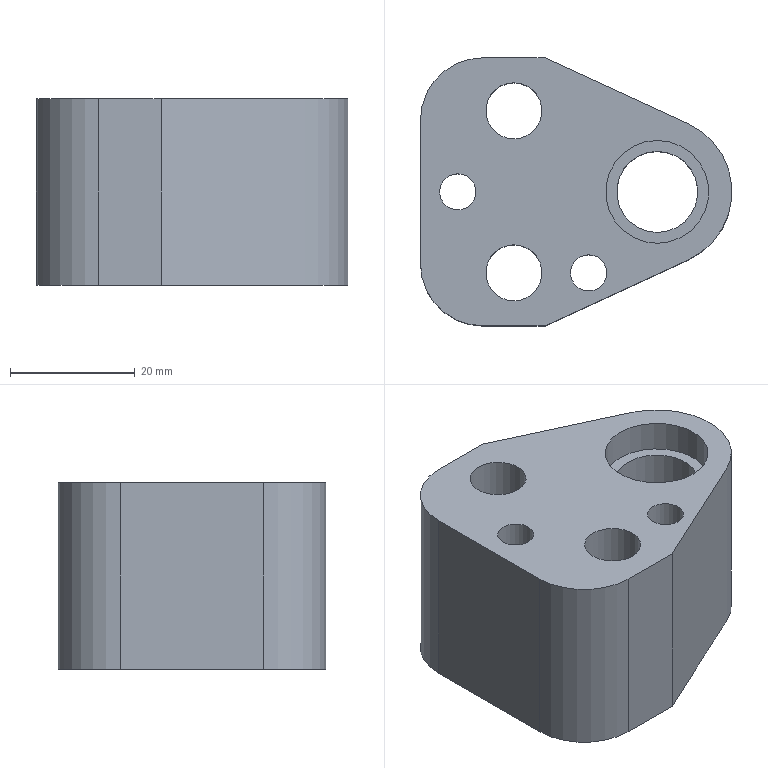Part | NX | features solid 2 | 1 solid | 27 faces | box 50 x 43 x 30 mm | volume 37617 mm3 | plane 14 | cylinder 13 | commonest cylinder face diameters 5.8 x2 8 x2 9 x2 14 x2 20 x2 13 x1
STEP:
#1=CARTESIAN_POINT('',(344.165,-485.402,142.));
#2=VERTEX_POINT('',#1);
#3=CARTESIAN_POINT('',(344.165,-485.402,172.));
#4=VERTEX_POINT('',#3);
#5=CARTESIAN_POINT('',(344.165,-485.402,142.));
#6=DIRECTION('',(0.,0.,1.));
#7=VECTOR('',#6,1000.);
#8=LINE('',#5,#7);
#9=EDGE_CURVE('',#2,#4,#8,.T.);
#10=ORIENTED_EDGE('',*,*,#9,.F.);
#11=CARTESIAN_POINT('',(344.165,-485.402,142.));
#12=VERTEX_POINT('',#11);
#13=CARTESIAN_POINT('',(344.165,-474.502,142.));
#14=DIRECTION('',(0.,1.,0.));
#15=VECTOR('',#14,1000.);
#16=LINE('',#13,#15);
#17=EDGE_CURVE('',#2,#12,#16,.T.);
#18=ORIENTED_EDGE('',*,*,#17,.T.);
#19=CARTESIAN_POINT('',(344.165,-485.402,172.));
#20=VERTEX_POINT('',#19);
#21=CARTESIAN_POINT('',(344.165,-485.402,172.));
#22=DIRECTION('',(0.,0.,-1.));
#23=VECTOR('',#22,1000.);
#24=LINE('',#21,#23);
#25=EDGE_CURVE('',#20,#12,#24,.T.);
#26=ORIENTED_EDGE('',*,*,#25,.F.);
#27=CARTESIAN_POINT('',(344.165,-474.502,172.));
#28=DIRECTION('',(0.,-1.,0.));
#29=VECTOR('',#28,1000.);
#30=LINE('',#27,#29);
#31=EDGE_CURVE('',#20,#4,#30,.T.);
#32=ORIENTED_EDGE('',*,*,#31,.T.);
#33=EDGE_LOOP('',(#10,#18,#26,#32));
#34=FACE_BOUND('',#33,.T.);
#35=CARTESIAN_POINT('',(344.165,-474.502,142.));
#36=DIRECTION('',(1.,0.,0.));
#37=DIRECTION('',(0.,0.,1.));
#38=AXIS2_PLACEMENT_3D('',#35,#36,#37);
#39=PLANE('',#38);
#40=ADVANCED_FACE('',(#34),#39,.T.);
#41=CARTESIAN_POINT('',(321.145,-496.002,172.));
#42=VERTEX_POINT('',#41);
#43=CARTESIAN_POINT('',(339.311,-487.637,172.));
#44=DIRECTION('',(0.9083,0.4183,0.));
#45=VECTOR('',#44,1000.);
#46=LINE('',#43,#45);
#47=EDGE_CURVE('',#42,#4,#46,.T.);
#48=ORIENTED_EDGE('',*,*,#47,.T.);
#49=ORIENTED_EDGE('',*,*,#31,.F.);
#50=CARTESIAN_POINT('',(344.165,-463.603,172.));
#51=VERTEX_POINT('',#50);
#52=CARTESIAN_POINT('',(339.145,-474.502,172.));
#53=DIRECTION('',(0.,0.,-1.));
#54=DIRECTION('',(0.,1.,0.));
#55=AXIS2_PLACEMENT_3D('',#52,#53,#54);
#56=CIRCLE('',#55,12.);
#57=EDGE_CURVE('',#51,#20,#56,.T.);
#58=ORIENTED_EDGE('',*,*,#57,.F.);
#59=CARTESIAN_POINT('',(344.165,-463.603,172.));
#60=VERTEX_POINT('',#59);
#61=CARTESIAN_POINT('',(344.165,-474.502,172.));
#62=DIRECTION('',(0.,-1.,0.));
#63=VECTOR('',#62,1000.);
#64=LINE('',#61,#63);
#65=EDGE_CURVE('',#60,#51,#64,.T.);
#66=ORIENTED_EDGE('',*,*,#65,.F.);
#67=CARTESIAN_POINT('',(321.145,-453.002,172.));
#68=VERTEX_POINT('',#67);
#69=CARTESIAN_POINT('',(339.311,-461.368,172.));
#70=DIRECTION('',(-0.9083,0.4183,0.));
#71=VECTOR('',#70,1000.);
#72=LINE('',#69,#71);
#73=EDGE_CURVE('',#60,#68,#72,.T.);
#74=ORIENTED_EDGE('',*,*,#73,.T.);
#75=CARTESIAN_POINT('',(311.145,-453.002,172.));
#76=VERTEX_POINT('',#75);
#77=CARTESIAN_POINT('',(332.655,-453.002,172.));
#78=DIRECTION('',(1.,0.,0.));
#79=VECTOR('',#78,1000.);
#80=LINE('',#77,#79);
#81=EDGE_CURVE('',#76,#68,#80,.T.);
#82=ORIENTED_EDGE('',*,*,#81,.F.);
#83=CARTESIAN_POINT('',(301.145,-463.002,172.));
#84=VERTEX_POINT('',#83);
#85=CARTESIAN_POINT('',(311.145,-463.002,172.));
#86=DIRECTION('',(0.,0.,1.));
#87=DIRECTION('',(0.,-1.,0.));
#88=AXIS2_PLACEMENT_3D('',#85,#86,#87);
#89=CIRCLE('',#88,10.);
#90=EDGE_CURVE('',#76,#84,#89,.T.);
#91=ORIENTED_EDGE('',*,*,#90,.T.);
#92=CARTESIAN_POINT('',(301.145,-486.002,172.));
#93=VERTEX_POINT('',#92);
#94=CARTESIAN_POINT('',(301.145,-474.502,172.));
#95=DIRECTION('',(0.,1.,0.));
#96=VECTOR('',#95,1000.);
#97=LINE('',#94,#96);
#98=EDGE_CURVE('',#93,#84,#97,.T.);
#99=ORIENTED_EDGE('',*,*,#98,.F.);
#100=CARTESIAN_POINT('',(311.145,-496.002,172.));
#101=VERTEX_POINT('',#100);
#102=CARTESIAN_POINT('',(311.145,-486.002,172.));
#103=DIRECTION('',(0.,0.,1.));
#104=DIRECTION('',(0.,-1.,0.));
#105=AXIS2_PLACEMENT_3D('',#102,#103,#104);
#106=CIRCLE('',#105,10.);
#107=EDGE_CURVE('',#93,#101,#106,.T.);
#108=ORIENTED_EDGE('',*,*,#107,.T.);
#109=CARTESIAN_POINT('',(332.655,-496.002,172.));
#110=DIRECTION('',(-1.,0.,0.));
#111=VECTOR('',#110,1000.);
#112=LINE('',#109,#111);
#113=EDGE_CURVE('',#42,#101,#112,.T.);
#114=ORIENTED_EDGE('',*,*,#113,.F.);
#115=EDGE_LOOP('',(#48,#49,#58,#66,#74,#82,#91,#99,#108,#114));
#116=FACE_BOUND('',#115,.T.);
#117=CARTESIAN_POINT('',(307.145,-471.602,172.));
#118=VERTEX_POINT('',#117);
#119=CARTESIAN_POINT('',(307.145,-474.502,172.));
#120=DIRECTION('',(0.,0.,-1.));
#121=DIRECTION('',(0.,1.,0.));
#122=AXIS2_PLACEMENT_3D('',#119,#120,#121);
#123=CIRCLE('',#122,2.9);
#124=EDGE_CURVE('',#118,#118,#123,.T.);
#125=ORIENTED_EDGE('',*,*,#124,.T.);
#126=EDGE_LOOP('',(#125));
#127=FACE_BOUND('',#126,.T.);
#128=CARTESIAN_POINT('',(328.145,-484.602,172.));
#129=VERTEX_POINT('',#128);
#130=CARTESIAN_POINT('',(328.145,-487.502,172.));
#131=DIRECTION('',(0.,0.,-1.));
#132=DIRECTION('',(0.,1.,0.));
#133=AXIS2_PLACEMENT_3D('',#130,#131,#132);
#134=CIRCLE('',#133,2.9);
#135=EDGE_CURVE('',#129,#129,#134,.T.);
#136=ORIENTED_EDGE('',*,*,#135,.T.);
#137=EDGE_LOOP('',(#136));
#138=FACE_BOUND('',#137,.T.);
#139=CARTESIAN_POINT('',(316.145,-483.002,172.));
#140=VERTEX_POINT('',#139);
#141=CARTESIAN_POINT('',(316.145,-487.502,172.));
#142=DIRECTION('',(0.,0.,-1.));
#143=DIRECTION('',(0.,1.,0.));
#144=AXIS2_PLACEMENT_3D('',#141,#142,#143);
#145=CIRCLE('',#144,4.5);
#146=EDGE_CURVE('',#140,#140,#145,.T.);
#147=ORIENTED_EDGE('',*,*,#146,.T.);
#148=EDGE_LOOP('',(#147));
#149=FACE_BOUND('',#148,.T.);
#150=CARTESIAN_POINT('',(316.145,-457.002,172.));
#151=VERTEX_POINT('',#150);
#152=CARTESIAN_POINT('',(316.145,-461.502,172.));
#153=DIRECTION('',(0.,0.,-1.));
#154=DIRECTION('',(0.,1.,0.));
#155=AXIS2_PLACEMENT_3D('',#152,#153,#154);
#156=CIRCLE('',#155,4.5);
#157=EDGE_CURVE('',#151,#151,#156,.T.);
#158=ORIENTED_EDGE('',*,*,#157,.T.);
#159=EDGE_LOOP('',(#158));
#160=FACE_BOUND('',#159,.T.);
#161=CARTESIAN_POINT('',(339.145,-466.252,172.));
#162=VERTEX_POINT('',#161);
#163=CARTESIAN_POINT('',(339.145,-474.502,172.));
#164=DIRECTION('',(0.,0.,-1.));
#165=DIRECTION('',(0.,1.,0.));
#166=AXIS2_PLACEMENT_3D('',#163,#164,#165);
#167=CIRCLE('',#166,8.25);
#168=EDGE_CURVE('',#162,#162,#167,.T.);
#169=ORIENTED_EDGE('',*,*,#168,.T.);
#170=EDGE_LOOP('',(#169));
#171=FACE_BOUND('',#170,.T.);
#172=CARTESIAN_POINT('',(332.655,-474.502,172.));
#173=DIRECTION('',(0.,0.,1.));
#174=DIRECTION('',(0.,-1.,0.));
#175=AXIS2_PLACEMENT_3D('',#172,#173,#174);
#176=PLANE('',#175);
#177=ADVANCED_FACE('',(#116,#127,#138,#149,#160,#171),#176,.T.);
#178=CARTESIAN_POINT('',(321.145,-453.002,142.));
#179=VERTEX_POINT('',#178);
#180=CARTESIAN_POINT('',(321.145,-453.002,142.));
#181=DIRECTION('',(0.,0.,1.));
#182=VECTOR('',#181,1000.);
#183=LINE('',#180,#182);
#184=EDGE_CURVE('',#179,#68,#183,.T.);
#185=ORIENTED_EDGE('',*,*,#184,.F.);
#186=CARTESIAN_POINT('',(311.145,-453.002,142.));
#187=VERTEX_POINT('',#186);
#188=CARTESIAN_POINT('',(332.655,-453.002,142.));
#189=DIRECTION('',(-1.,0.,0.));
#190=VECTOR('',#189,1000.);
#191=LINE('',#188,#190);
#192=EDGE_CURVE('',#179,#187,#191,.T.);
#193=ORIENTED_EDGE('',*,*,#192,.T.);
#194=CARTESIAN_POINT('',(311.145,-453.002,142.));
#195=DIRECTION('',(0.,0.,1.));
#196=VECTOR('',#195,1000.);
#197=LINE('',#194,#196);
#198=EDGE_CURVE('',#187,#76,#197,.T.);
#199=ORIENTED_EDGE('',*,*,#198,.T.);
#200=ORIENTED_EDGE('',*,*,#81,.T.);
#201=EDGE_LOOP('',(#185,#193,#199,#200));
#202=FACE_BOUND('',#201,.T.);
#203=CARTESIAN_POINT('',(332.655,-453.002,142.));
#204=DIRECTION('',(0.,1.,0.));
#205=DIRECTION('',(0.,0.,1.));
#206=AXIS2_PLACEMENT_3D('',#203,#204,#205);
#207=PLANE('',#206);
#208=ADVANCED_FACE('',(#202),#207,.T.);
#209=CARTESIAN_POINT('',(344.165,-463.603,142.));
#210=VERTEX_POINT('',#209);
#211=CARTESIAN_POINT('',(344.165,-463.603,142.));
#212=DIRECTION('',(0.,0.,-1.));
#213=VECTOR('',#212,1000.);
#214=LINE('',#211,#213);
#215=EDGE_CURVE('',#60,#210,#214,.T.);
#216=ORIENTED_EDGE('',*,*,#215,.F.);
#217=ORIENTED_EDGE('',*,*,#65,.T.);
#218=CARTESIAN_POINT('',(344.165,-463.603,142.));
#219=VERTEX_POINT('',#218);
#220=CARTESIAN_POINT('',(344.165,-463.603,172.));
#221=DIRECTION('',(0.,0.,-1.));
#222=VECTOR('',#221,1000.);
#223=LINE('',#220,#222);
#224=EDGE_CURVE('',#219,#51,#223,.F.);
#225=ORIENTED_EDGE('',*,*,#224,.F.);
#226=CARTESIAN_POINT('',(344.165,-474.502,142.));
#227=DIRECTION('',(0.,1.,0.));
#228=VECTOR('',#227,1000.);
#229=LINE('',#226,#228);
#230=EDGE_CURVE('',#219,#210,#229,.T.);
#231=ORIENTED_EDGE('',*,*,#230,.T.);
#232=EDGE_LOOP('',(#216,#217,#225,#231));
#233=FACE_BOUND('',#232,.T.);
#234=CARTESIAN_POINT('',(344.165,-474.502,142.));
#235=DIRECTION('',(1.,0.,0.));
#236=DIRECTION('',(0.,0.,1.));
#237=AXIS2_PLACEMENT_3D('',#234,#235,#236);
#238=PLANE('',#237);
#239=ADVANCED_FACE('',(#233),#238,.T.);
#240=CARTESIAN_POINT('',(321.145,-496.002,142.));
#241=VERTEX_POINT('',#240);
#242=CARTESIAN_POINT('',(339.311,-487.637,142.));
#243=DIRECTION('',(-0.9083,-0.4183,0.));
#244=VECTOR('',#243,1000.);
#245=LINE('',#242,#244);
#246=EDGE_CURVE('',#2,#241,#245,.T.);
#247=ORIENTED_EDGE('',*,*,#246,.T.);
#248=CARTESIAN_POINT('',(311.145,-496.002,142.));
#249=VERTEX_POINT('',#248);
#250=CARTESIAN_POINT('',(332.655,-496.002,142.));
#251=DIRECTION('',(1.,0.,0.));
#252=VECTOR('',#251,1000.);
#253=LINE('',#250,#252);
#254=EDGE_CURVE('',#249,#241,#253,.T.);
#255=ORIENTED_EDGE('',*,*,#254,.F.);
#256=CARTESIAN_POINT('',(301.145,-486.002,142.));
#257=VERTEX_POINT('',#256);
#258=CARTESIAN_POINT('',(311.145,-486.002,142.));
#259=DIRECTION('',(0.,0.,-1.));
#260=DIRECTION('',(0.,1.,0.));
#261=AXIS2_PLACEMENT_3D('',#258,#259,#260);
#262=CIRCLE('',#261,10.);
#263=EDGE_CURVE('',#249,#257,#262,.T.);
#264=ORIENTED_EDGE('',*,*,#263,.T.);
#265=CARTESIAN_POINT('',(301.145,-463.002,142.));
#266=VERTEX_POINT('',#265);
#267=CARTESIAN_POINT('',(301.145,-474.502,142.));
#268=DIRECTION('',(0.,-1.,0.));
#269=VECTOR('',#268,1000.);
#270=LINE('',#267,#269);
#271=EDGE_CURVE('',#266,#257,#270,.T.);
#272=ORIENTED_EDGE('',*,*,#271,.F.);
#273=CARTESIAN_POINT('',(311.145,-463.002,142.));
#274=DIRECTION('',(0.,0.,-1.));
#275=DIRECTION('',(0.,1.,0.));
#276=AXIS2_PLACEMENT_3D('',#273,#274,#275);
#277=CIRCLE('',#276,10.);
#278=EDGE_CURVE('',#266,#187,#277,.T.);
#279=ORIENTED_EDGE('',*,*,#278,.T.);
#280=ORIENTED_EDGE('',*,*,#192,.F.);
#281=CARTESIAN_POINT('',(339.311,-461.368,142.));
#282=DIRECTION('',(0.9083,-0.4183,0.));
#283=VECTOR('',#282,1000.);
#284=LINE('',#281,#283);
#285=EDGE_CURVE('',#179,#210,#284,.T.);
#286=ORIENTED_EDGE('',*,*,#285,.T.);
#287=ORIENTED_EDGE('',*,*,#230,.F.);
#288=CARTESIAN_POINT('',(339.145,-474.502,142.));
#289=DIRECTION('',(0.,0.,1.));
#290=DIRECTION('',(0.,-1.,0.));
#291=AXIS2_PLACEMENT_3D('',#288,#289,#290);
#292=CIRCLE('',#291,12.);
#293=EDGE_CURVE('',#12,#219,#292,.T.);
#294=ORIENTED_EDGE('',*,*,#293,.F.);
#295=ORIENTED_EDGE('',*,*,#17,.F.);
#296=EDGE_LOOP('',(#247,#255,#264,#272,#279,#280,#286,#287,#294,#295));
#297=FACE_BOUND('',#296,.T.);
#298=CARTESIAN_POINT('',(307.145,-478.502,142.));
#299=VERTEX_POINT('',#298);
#300=CARTESIAN_POINT('',(307.145,-474.502,142.));
#301=DIRECTION('',(0.,0.,1.));
#302=DIRECTION('',(0.,-1.,0.));
#303=AXIS2_PLACEMENT_3D('',#300,#301,#302);
#304=CIRCLE('',#303,4.);
#305=EDGE_CURVE('',#299,#299,#304,.T.);
#306=ORIENTED_EDGE('',*,*,#305,.T.);
#307=EDGE_LOOP('',(#306));
#308=FACE_BOUND('',#307,.T.);
#309=CARTESIAN_POINT('',(328.145,-491.502,142.));
#310=VERTEX_POINT('',#309);
#311=CARTESIAN_POINT('',(328.145,-487.502,142.));
#312=DIRECTION('',(0.,0.,1.));
#313=DIRECTION('',(0.,-1.,0.));
#314=AXIS2_PLACEMENT_3D('',#311,#312,#313);
#315=CIRCLE('',#314,4.);
#316=EDGE_CURVE('',#310,#310,#315,.T.);
#317=ORIENTED_EDGE('',*,*,#316,.T.);
#318=EDGE_LOOP('',(#317));
#319=FACE_BOUND('',#318,.T.);
#320=CARTESIAN_POINT('',(316.145,-494.502,142.));
#321=VERTEX_POINT('',#320);
#322=CARTESIAN_POINT('',(316.145,-487.502,142.));
#323=DIRECTION('',(0.,0.,1.));
#324=DIRECTION('',(0.,-1.,0.));
#325=AXIS2_PLACEMENT_3D('',#322,#323,#324);
#326=CIRCLE('',#325,7.);
#327=EDGE_CURVE('',#321,#321,#326,.T.);
#328=ORIENTED_EDGE('',*,*,#327,.T.);
#329=EDGE_LOOP('',(#328));
#330=FACE_BOUND('',#329,.T.);
#331=CARTESIAN_POINT('',(316.145,-468.502,142.));
#332=VERTEX_POINT('',#331);
#333=CARTESIAN_POINT('',(316.145,-461.502,142.));
#334=DIRECTION('',(0.,0.,1.));
#335=DIRECTION('',(0.,-1.,0.));
#336=AXIS2_PLACEMENT_3D('',#333,#334,#335);
#337=CIRCLE('',#336,7.);
#338=EDGE_CURVE('',#332,#332,#337,.T.);
#339=ORIENTED_EDGE('',*,*,#338,.T.);
#340=EDGE_LOOP('',(#339));
#341=FACE_BOUND('',#340,.T.);
#342=CARTESIAN_POINT('',(339.145,-481.002,142.));
#343=VERTEX_POINT('',#342);
#344=CARTESIAN_POINT('',(339.145,-474.502,142.));
#345=DIRECTION('',(0.,0.,1.));
#346=DIRECTION('',(0.,-1.,0.));
#347=AXIS2_PLACEMENT_3D('',#344,#345,#346);
#348=CIRCLE('',#347,6.5);
#349=EDGE_CURVE('',#343,#343,#348,.T.);
#350=ORIENTED_EDGE('',*,*,#349,.T.);
#351=EDGE_LOOP('',(#350));
#352=FACE_BOUND('',#351,.T.);
#353=CARTESIAN_POINT('',(332.655,-474.502,142.));
#354=DIRECTION('',(0.,0.,-1.));
#355=DIRECTION('',(0.,1.,0.));
#356=AXIS2_PLACEMENT_3D('',#353,#354,#355);
#357=PLANE('',#356);
#358=ADVANCED_FACE('',(#297,#308,#319,#330,#341,#352),#357,.T.);
#359=CARTESIAN_POINT('',(321.145,-496.002,142.));
#360=DIRECTION('',(0.,0.,1.));
#361=VECTOR('',#360,1000.);
#362=LINE('',#359,#361);
#363=EDGE_CURVE('',#241,#42,#362,.T.);
#364=ORIENTED_EDGE('',*,*,#363,.T.);
#365=ORIENTED_EDGE('',*,*,#113,.T.);
#366=CARTESIAN_POINT('',(311.145,-496.002,142.));
#367=DIRECTION('',(0.,0.,1.));
#368=VECTOR('',#367,1000.);
#369=LINE('',#366,#368);
#370=EDGE_CURVE('',#101,#249,#369,.F.);
#371=ORIENTED_EDGE('',*,*,#370,.T.);
#372=ORIENTED_EDGE('',*,*,#254,.T.);
#373=EDGE_LOOP('',(#364,#365,#371,#372));
#374=FACE_BOUND('',#373,.T.);
#375=CARTESIAN_POINT('',(332.655,-496.002,142.));
#376=DIRECTION('',(0.,-1.,0.));
#377=DIRECTION('',(0.,0.,-1.));
#378=AXIS2_PLACEMENT_3D('',#375,#376,#377);
#379=PLANE('',#378);
#380=ADVANCED_FACE('',(#374),#379,.T.);
#381=ORIENTED_EDGE('',*,*,#57,.T.);
#382=ORIENTED_EDGE('',*,*,#25,.T.);
#383=ORIENTED_EDGE('',*,*,#293,.T.);
#384=ORIENTED_EDGE('',*,*,#224,.T.);
#385=EDGE_LOOP('',(#381,#382,#383,#384));
#386=FACE_BOUND('',#385,.T.);
#387=CARTESIAN_POINT('',(339.145,-474.502,172.));
#388=DIRECTION('',(0.,0.,-1.));
#389=DIRECTION('',(0.,1.,0.));
#390=AXIS2_PLACEMENT_3D('',#387,#388,#389);
#391=CYLINDRICAL_SURFACE('',#390,12.);
#392=ADVANCED_FACE('',(#386),#391,.T.);
#393=ORIENTED_EDGE('',*,*,#271,.T.);
#394=CARTESIAN_POINT('',(301.145,-486.002,142.));
#395=DIRECTION('',(0.,0.,1.));
#396=VECTOR('',#395,1000.);
#397=LINE('',#394,#396);
#398=EDGE_CURVE('',#257,#93,#397,.T.);
#399=ORIENTED_EDGE('',*,*,#398,.T.);
#400=ORIENTED_EDGE('',*,*,#98,.T.);
#401=CARTESIAN_POINT('',(301.145,-463.002,142.));
#402=DIRECTION('',(0.,0.,1.));
#403=VECTOR('',#402,1000.);
#404=LINE('',#401,#403);
#405=EDGE_CURVE('',#84,#266,#404,.F.);
#406=ORIENTED_EDGE('',*,*,#405,.T.);
#407=EDGE_LOOP('',(#393,#399,#400,#406));
#408=FACE_BOUND('',#407,.T.);
#409=CARTESIAN_POINT('',(301.145,-474.502,142.));
#410=DIRECTION('',(-1.,0.,0.));
#411=DIRECTION('',(0.,0.,-1.));
#412=AXIS2_PLACEMENT_3D('',#409,#410,#411);
#413=PLANE('',#412);
#414=ADVANCED_FACE('',(#408),#413,.T.);
#415=CARTESIAN_POINT('',(339.145,-468.002,167.));
#416=VERTEX_POINT('',#415);
#417=CARTESIAN_POINT('',(339.145,-474.502,167.));
#418=DIRECTION('',(0.,0.,-1.));
#419=DIRECTION('',(0.,1.,0.));
#420=AXIS2_PLACEMENT_3D('',#417,#418,#419);
#421=CIRCLE('',#420,6.5);
#422=EDGE_CURVE('',#416,#416,#421,.T.);
#423=ORIENTED_EDGE('',*,*,#422,.T.);
#424=EDGE_LOOP('',(#423));
#425=FACE_BOUND('',#424,.T.);
#426=CARTESIAN_POINT('',(339.145,-482.752,167.));
#427=VERTEX_POINT('',#426);
#428=CARTESIAN_POINT('',(339.145,-474.502,167.));
#429=DIRECTION('',(0.,0.,1.));
#430=DIRECTION('',(0.,-1.,0.));
#431=AXIS2_PLACEMENT_3D('',#428,#429,#430);
#432=CIRCLE('',#431,8.25);
#433=EDGE_CURVE('',#427,#427,#432,.T.);
#434=ORIENTED_EDGE('',*,*,#433,.T.);
#435=EDGE_LOOP('',(#434));
#436=FACE_BOUND('',#435,.T.);
#437=CARTESIAN_POINT('',(339.145,-474.502,167.));
#438=DIRECTION('',(0.,0.,-1.));
#439=DIRECTION('',(0.,1.,0.));
#440=AXIS2_PLACEMENT_3D('',#437,#438,#439);
#441=PLANE('',#440);
#442=ADVANCED_FACE('',(#425,#436),#441,.F.);
#443=ORIENTED_EDGE('',*,*,#433,.F.);
#444=EDGE_LOOP('',(#443));
#445=FACE_BOUND('',#444,.T.);
#446=ORIENTED_EDGE('',*,*,#168,.F.);
#447=EDGE_LOOP('',(#446));
#448=FACE_BOUND('',#447,.T.);
#449=CARTESIAN_POINT('',(339.145,-474.502,172.));
#450=DIRECTION('',(0.,0.,-1.));
#451=DIRECTION('',(0.,1.,0.));
#452=AXIS2_PLACEMENT_3D('',#449,#450,#451);
#453=CYLINDRICAL_SURFACE('',#452,8.25);
#454=ADVANCED_FACE('',(#445,#448),#453,.F.);
#455=ORIENTED_EDGE('',*,*,#349,.F.);
#456=EDGE_LOOP('',(#455));
#457=FACE_BOUND('',#456,.T.);
#458=ORIENTED_EDGE('',*,*,#422,.F.);
#459=EDGE_LOOP('',(#458));
#460=FACE_BOUND('',#459,.T.);
#461=CARTESIAN_POINT('',(339.145,-474.502,167.));
#462=DIRECTION('',(0.,0.,-1.));
#463=DIRECTION('',(0.,1.,0.));
#464=AXIS2_PLACEMENT_3D('',#461,#462,#463);
#465=CYLINDRICAL_SURFACE('',#464,6.5);
#466=ADVANCED_FACE('',(#457,#460),#465,.F.);
#467=CARTESIAN_POINT('',(316.145,-466.002,152.));
#468=VERTEX_POINT('',#467);
#469=CARTESIAN_POINT('',(316.145,-461.502,152.));
#470=DIRECTION('',(0.,0.,1.));
#471=DIRECTION('',(0.,-1.,0.));
#472=AXIS2_PLACEMENT_3D('',#469,#470,#471);
#473=CIRCLE('',#472,4.5);
#474=EDGE_CURVE('',#468,#468,#473,.F.);
#475=ORIENTED_EDGE('',*,*,#474,.T.);
#476=EDGE_LOOP('',(#475));
#477=FACE_BOUND('',#476,.T.);
#478=ORIENTED_EDGE('',*,*,#157,.F.);
#479=EDGE_LOOP('',(#478));
#480=FACE_BOUND('',#479,.T.);
#481=CARTESIAN_POINT('',(316.145,-461.502,172.));
#482=DIRECTION('',(0.,0.,-1.));
#483=DIRECTION('',(0.,1.,0.));
#484=AXIS2_PLACEMENT_3D('',#481,#482,#483);
#485=CYLINDRICAL_SURFACE('',#484,4.5);
#486=ADVANCED_FACE('',(#477,#480),#485,.F.);
#487=CARTESIAN_POINT('',(316.145,-454.502,152.));
#488=VERTEX_POINT('',#487);
#489=CARTESIAN_POINT('',(316.145,-461.502,152.));
#490=DIRECTION('',(0.,0.,-1.));
#491=DIRECTION('',(0.,1.,0.));
#492=AXIS2_PLACEMENT_3D('',#489,#490,#491);
#493=CIRCLE('',#492,7.);
#494=EDGE_CURVE('',#488,#488,#493,.T.);
#495=ORIENTED_EDGE('',*,*,#494,.T.);
#496=EDGE_LOOP('',(#495));
#497=FACE_BOUND('',#496,.T.);
#498=ORIENTED_EDGE('',*,*,#474,.F.);
#499=EDGE_LOOP('',(#498));
#500=FACE_BOUND('',#499,.T.);
#501=CARTESIAN_POINT('',(316.145,-461.502,152.));
#502=DIRECTION('',(0.,0.,1.));
#503=DIRECTION('',(0.,-1.,0.));
#504=AXIS2_PLACEMENT_3D('',#501,#502,#503);
#505=PLANE('',#504);
#506=ADVANCED_FACE('',(#497,#500),#505,.F.);
#507=ORIENTED_EDGE('',*,*,#338,.F.);
#508=EDGE_LOOP('',(#507));
#509=FACE_BOUND('',#508,.T.);
#510=ORIENTED_EDGE('',*,*,#494,.F.);
#511=EDGE_LOOP('',(#510));
#512=FACE_BOUND('',#511,.T.);
#513=CARTESIAN_POINT('',(316.145,-461.502,152.));
#514=DIRECTION('',(0.,0.,-1.));
#515=DIRECTION('',(0.,1.,0.));
#516=AXIS2_PLACEMENT_3D('',#513,#514,#515);
#517=CYLINDRICAL_SURFACE('',#516,7.);
#518=ADVANCED_FACE('',(#509,#512),#517,.F.);
#519=CARTESIAN_POINT('',(316.145,-492.002,152.));
#520=VERTEX_POINT('',#519);
#521=CARTESIAN_POINT('',(316.145,-487.502,152.));
#522=DIRECTION('',(0.,0.,1.));
#523=DIRECTION('',(0.,-1.,0.));
#524=AXIS2_PLACEMENT_3D('',#521,#522,#523);
#525=CIRCLE('',#524,4.5);
#526=EDGE_CURVE('',#520,#520,#525,.F.);
#527=ORIENTED_EDGE('',*,*,#526,.T.);
#528=EDGE_LOOP('',(#527));
#529=FACE_BOUND('',#528,.T.);
#530=ORIENTED_EDGE('',*,*,#146,.F.);
#531=EDGE_LOOP('',(#530));
#532=FACE_BOUND('',#531,.T.);
#533=CARTESIAN_POINT('',(316.145,-487.502,172.));
#534=DIRECTION('',(0.,0.,-1.));
#535=DIRECTION('',(0.,1.,0.));
#536=AXIS2_PLACEMENT_3D('',#533,#534,#535);
#537=CYLINDRICAL_SURFACE('',#536,4.5);
#538=ADVANCED_FACE('',(#529,#532),#537,.F.);
#539=CARTESIAN_POINT('',(316.145,-480.502,152.));
#540=VERTEX_POINT('',#539);
#541=CARTESIAN_POINT('',(316.145,-487.502,152.));
#542=DIRECTION('',(0.,0.,-1.));
#543=DIRECTION('',(0.,1.,0.));
#544=AXIS2_PLACEMENT_3D('',#541,#542,#543);
#545=CIRCLE('',#544,7.);
#546=EDGE_CURVE('',#540,#540,#545,.T.);
#547=ORIENTED_EDGE('',*,*,#546,.T.);
#548=EDGE_LOOP('',(#547));
#549=FACE_BOUND('',#548,.T.);
#550=ORIENTED_EDGE('',*,*,#526,.F.);
#551=EDGE_LOOP('',(#550));
#552=FACE_BOUND('',#551,.T.);
#553=CARTESIAN_POINT('',(316.145,-487.502,152.));
#554=DIRECTION('',(0.,0.,1.));
#555=DIRECTION('',(0.,-1.,0.));
#556=AXIS2_PLACEMENT_3D('',#553,#554,#555);
#557=PLANE('',#556);
#558=ADVANCED_FACE('',(#549,#552),#557,.F.);
#559=ORIENTED_EDGE('',*,*,#327,.F.);
#560=EDGE_LOOP('',(#559));
#561=FACE_BOUND('',#560,.T.);
#562=ORIENTED_EDGE('',*,*,#546,.F.);
#563=EDGE_LOOP('',(#562));
#564=FACE_BOUND('',#563,.T.);
#565=CARTESIAN_POINT('',(316.145,-487.502,152.));
#566=DIRECTION('',(0.,0.,-1.));
#567=DIRECTION('',(0.,1.,0.));
#568=AXIS2_PLACEMENT_3D('',#565,#566,#567);
#569=CYLINDRICAL_SURFACE('',#568,7.);
#570=ADVANCED_FACE('',(#561,#564),#569,.F.);
#571=CARTESIAN_POINT('',(328.145,-490.402,162.));
#572=VERTEX_POINT('',#571);
#573=CARTESIAN_POINT('',(328.145,-487.502,162.));
#574=DIRECTION('',(0.,0.,1.));
#575=DIRECTION('',(0.,-1.,0.));
#576=AXIS2_PLACEMENT_3D('',#573,#574,#575);
#577=CIRCLE('',#576,2.9);
#578=EDGE_CURVE('',#572,#572,#577,.F.);
#579=ORIENTED_EDGE('',*,*,#578,.T.);
#580=EDGE_LOOP('',(#579));
#581=FACE_BOUND('',#580,.T.);
#582=ORIENTED_EDGE('',*,*,#135,.F.);
#583=EDGE_LOOP('',(#582));
#584=FACE_BOUND('',#583,.T.);
#585=CARTESIAN_POINT('',(328.145,-487.502,172.));
#586=DIRECTION('',(0.,0.,-1.));
#587=DIRECTION('',(0.,1.,0.));
#588=AXIS2_PLACEMENT_3D('',#585,#586,#587);
#589=CYLINDRICAL_SURFACE('',#588,2.9);
#590=ADVANCED_FACE('',(#581,#584),#589,.F.);
#591=CARTESIAN_POINT('',(328.145,-483.502,162.));
#592=VERTEX_POINT('',#591);
#593=CARTESIAN_POINT('',(328.145,-487.502,162.));
#594=DIRECTION('',(0.,0.,-1.));
#595=DIRECTION('',(0.,1.,0.));
#596=AXIS2_PLACEMENT_3D('',#593,#594,#595);
#597=CIRCLE('',#596,4.);
#598=EDGE_CURVE('',#592,#592,#597,.T.);
#599=ORIENTED_EDGE('',*,*,#598,.T.);
#600=EDGE_LOOP('',(#599));
#601=FACE_BOUND('',#600,.T.);
#602=ORIENTED_EDGE('',*,*,#578,.F.);
#603=EDGE_LOOP('',(#602));
#604=FACE_BOUND('',#603,.T.);
#605=CARTESIAN_POINT('',(328.145,-487.502,162.));
#606=DIRECTION('',(0.,0.,1.));
#607=DIRECTION('',(0.,-1.,0.));
#608=AXIS2_PLACEMENT_3D('',#605,#606,#607);
#609=PLANE('',#608);
#610=ADVANCED_FACE('',(#601,#604),#609,.F.);
#611=ORIENTED_EDGE('',*,*,#316,.F.);
#612=EDGE_LOOP('',(#611));
#613=FACE_BOUND('',#612,.T.);
#614=ORIENTED_EDGE('',*,*,#598,.F.);
#615=EDGE_LOOP('',(#614));
#616=FACE_BOUND('',#615,.T.);
#617=CARTESIAN_POINT('',(328.145,-487.502,162.));
#618=DIRECTION('',(0.,0.,-1.));
#619=DIRECTION('',(0.,1.,0.));
#620=AXIS2_PLACEMENT_3D('',#617,#618,#619);
#621=CYLINDRICAL_SURFACE('',#620,4.);
#622=ADVANCED_FACE('',(#613,#616),#621,.F.);
#623=CARTESIAN_POINT('',(307.145,-477.402,162.));
#624=VERTEX_POINT('',#623);
#625=CARTESIAN_POINT('',(307.145,-474.502,162.));
#626=DIRECTION('',(0.,0.,1.));
#627=DIRECTION('',(0.,-1.,0.));
#628=AXIS2_PLACEMENT_3D('',#625,#626,#627);
#629=CIRCLE('',#628,2.9);
#630=EDGE_CURVE('',#624,#624,#629,.F.);
#631=ORIENTED_EDGE('',*,*,#630,.T.);
#632=EDGE_LOOP('',(#631));
#633=FACE_BOUND('',#632,.T.);
#634=ORIENTED_EDGE('',*,*,#124,.F.);
#635=EDGE_LOOP('',(#634));
#636=FACE_BOUND('',#635,.T.);
#637=CARTESIAN_POINT('',(307.145,-474.502,172.));
#638=DIRECTION('',(0.,0.,-1.));
#639=DIRECTION('',(0.,1.,0.));
#640=AXIS2_PLACEMENT_3D('',#637,#638,#639);
#641=CYLINDRICAL_SURFACE('',#640,2.9);
#642=ADVANCED_FACE('',(#633,#636),#641,.F.);
#643=CARTESIAN_POINT('',(307.145,-470.502,162.));
#644=VERTEX_POINT('',#643);
#645=CARTESIAN_POINT('',(307.145,-474.502,162.));
#646=DIRECTION('',(0.,0.,-1.));
#647=DIRECTION('',(0.,1.,0.));
#648=AXIS2_PLACEMENT_3D('',#645,#646,#647);
#649=CIRCLE('',#648,4.);
#650=EDGE_CURVE('',#644,#644,#649,.T.);
#651=ORIENTED_EDGE('',*,*,#650,.T.);
#652=EDGE_LOOP('',(#651));
#653=FACE_BOUND('',#652,.T.);
#654=ORIENTED_EDGE('',*,*,#630,.F.);
#655=EDGE_LOOP('',(#654));
#656=FACE_BOUND('',#655,.T.);
#657=CARTESIAN_POINT('',(307.145,-474.502,162.));
#658=DIRECTION('',(0.,0.,1.));
#659=DIRECTION('',(0.,-1.,0.));
#660=AXIS2_PLACEMENT_3D('',#657,#658,#659);
#661=PLANE('',#660);
#662=ADVANCED_FACE('',(#653,#656),#661,.F.);
#663=ORIENTED_EDGE('',*,*,#305,.F.);
#664=EDGE_LOOP('',(#663));
#665=FACE_BOUND('',#664,.T.);
#666=ORIENTED_EDGE('',*,*,#650,.F.);
#667=EDGE_LOOP('',(#666));
#668=FACE_BOUND('',#667,.T.);
#669=CARTESIAN_POINT('',(307.145,-474.502,162.));
#670=DIRECTION('',(0.,0.,-1.));
#671=DIRECTION('',(0.,1.,0.));
#672=AXIS2_PLACEMENT_3D('',#669,#670,#671);
#673=CYLINDRICAL_SURFACE('',#672,4.);
#674=ADVANCED_FACE('',(#665,#668),#673,.F.);
#675=ORIENTED_EDGE('',*,*,#263,.F.);
#676=ORIENTED_EDGE('',*,*,#370,.F.);
#677=ORIENTED_EDGE('',*,*,#107,.F.);
#678=ORIENTED_EDGE('',*,*,#398,.F.);
#679=EDGE_LOOP('',(#675,#676,#677,#678));
#680=FACE_BOUND('',#679,.T.);
#681=CARTESIAN_POINT('',(311.145,-486.002,142.));
#682=DIRECTION('',(0.,0.,1.));
#683=DIRECTION('',(0.,-1.,0.));
#684=AXIS2_PLACEMENT_3D('',#681,#682,#683);
#685=CYLINDRICAL_SURFACE('',#684,10.);
#686=ADVANCED_FACE('',(#680),#685,.T.);
#687=ORIENTED_EDGE('',*,*,#278,.F.);
#688=ORIENTED_EDGE('',*,*,#405,.F.);
#689=ORIENTED_EDGE('',*,*,#90,.F.);
#690=ORIENTED_EDGE('',*,*,#198,.F.);
#691=EDGE_LOOP('',(#687,#688,#689,#690));
#692=FACE_BOUND('',#691,.T.);
#693=CARTESIAN_POINT('',(311.145,-463.002,142.));
#694=DIRECTION('',(0.,0.,1.));
#695=DIRECTION('',(0.,-1.,0.));
#696=AXIS2_PLACEMENT_3D('',#693,#694,#695);
#697=CYLINDRICAL_SURFACE('',#696,10.);
#698=ADVANCED_FACE('',(#692),#697,.T.);
#699=ORIENTED_EDGE('',*,*,#215,.T.);
#700=ORIENTED_EDGE('',*,*,#285,.F.);
#701=ORIENTED_EDGE('',*,*,#184,.T.);
#702=ORIENTED_EDGE('',*,*,#73,.F.);
#703=EDGE_LOOP('',(#699,#700,#701,#702));
#704=FACE_BOUND('',#703,.T.);
#705=CARTESIAN_POINT('',(339.311,-461.368,142.));
#706=DIRECTION('',(-0.4183,-0.9083,0.));
#707=DIRECTION('',(0.,0.,-1.));
#708=AXIS2_PLACEMENT_3D('',#705,#706,#707);
#709=PLANE('',#708);
#710=ADVANCED_FACE('',(#704),#709,.F.);
#711=ORIENTED_EDGE('',*,*,#9,.T.);
#712=ORIENTED_EDGE('',*,*,#47,.F.);
#713=ORIENTED_EDGE('',*,*,#363,.F.);
#714=ORIENTED_EDGE('',*,*,#246,.F.);
#715=EDGE_LOOP('',(#711,#712,#713,#714));
#716=FACE_BOUND('',#715,.T.);
#717=CARTESIAN_POINT('',(339.311,-487.637,142.));
#718=DIRECTION('',(-0.4183,0.9083,0.));
#719=DIRECTION('',(0.,0.,1.));
#720=AXIS2_PLACEMENT_3D('',#717,#718,#719);
#721=PLANE('',#720);
#722=ADVANCED_FACE('',(#716),#721,.F.);
#723=CLOSED_SHELL('',(#40,#177,#208,#239,#358,#380,#392,#414,#442,#454,#466,#486,#506,#518,#538,#558,#570,#590,#610,#622,#642,#662,#674,#686,#698,#710,#722));
#724=MANIFOLD_SOLID_BREP('',#723);
#725=(LENGTH_UNIT()NAMED_UNIT(*)SI_UNIT(.MILLI.,.METRE.));
#726=UNCERTAINTY_MEASURE_WITH_UNIT(LENGTH_MEASURE(0.00001),#725,'','');
#727=(NAMED_UNIT(*)PLANE_ANGLE_UNIT()SI_UNIT($,.RADIAN.));
#728=(NAMED_UNIT(*)SI_UNIT($,.STERADIAN.)SOLID_ANGLE_UNIT());
#729=(GEOMETRIC_REPRESENTATION_CONTEXT(3)GLOBAL_UNCERTAINTY_ASSIGNED_CONTEXT((#726))GLOBAL_UNIT_ASSIGNED_CONTEXT((#725,#727,#728))REPRESENTATION_CONTEXT('',''));
#730=ADVANCED_BREP_SHAPE_REPRESENTATION('',(#724),#729);